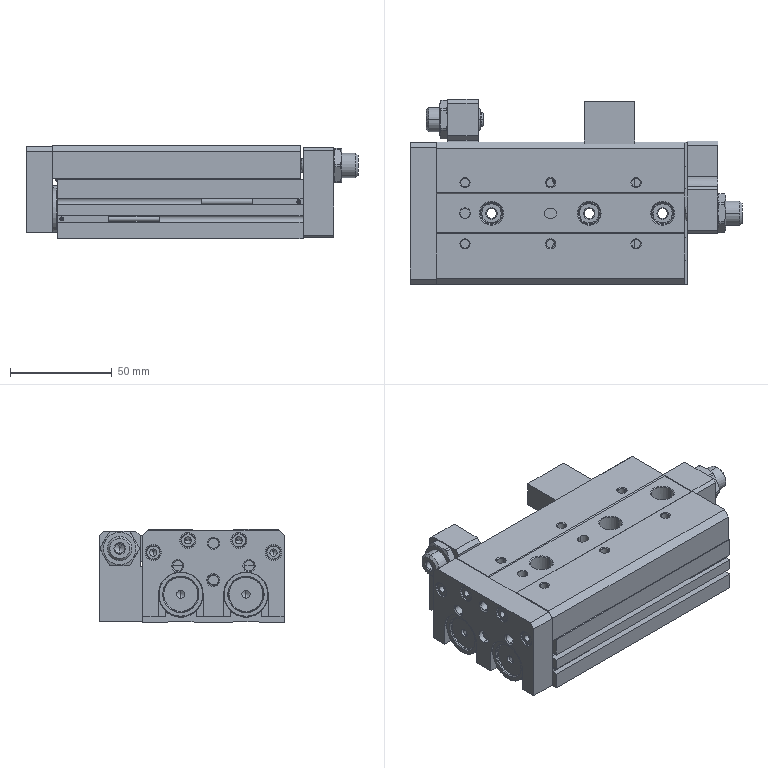Part | SolidWorks | features BaseBody 4 | 4 solids | 758 faces | box 163 x 91 x 46 mm | volume 387312 mm3 | plane 292 | cylinder 266 | cone 170 | spline 30 | commonest cylinder face diameters 4.917 x21 4.134 x20 7.5 x16 20 x14 3 x12 7 x12